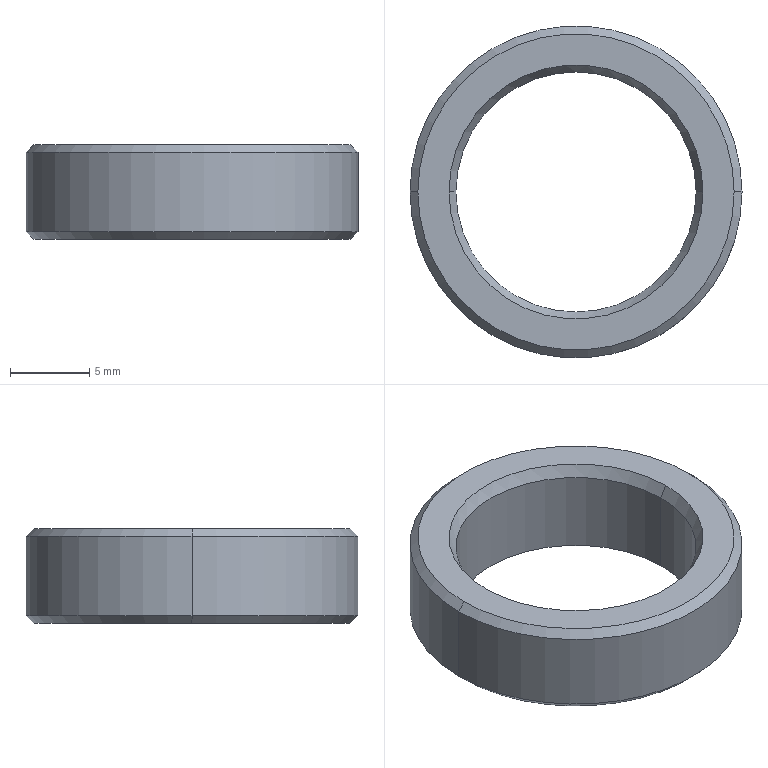Part | STEP file | ESPACIADOR POLEA 2 | 1 solid | 12 faces | box 21 x 21 x 6 mm | volume 965.28 mm3 | cone 6 | cylinder 4 | plane 2 | commonest cylinder face diameters 15.2 x2 21 x2
STEP:
#1=CARTESIAN_POINT('',(-7.6,0.,2.25));
#2=VERTEX_POINT('',#1);
#3=CARTESIAN_POINT('',(7.6,0.,2.25));
#4=VERTEX_POINT('',#3);
#5=CARTESIAN_POINT('',(0.,0.,2.25));
#6=DIRECTION('',(0.,0.,1.));
#7=DIRECTION('',(1.,0.,0.));
#8=AXIS2_PLACEMENT_3D('',#5,#6,#7);
#9=CIRCLE('',#8,7.6);
#10=EDGE_CURVE('',#2,#4,#9,.T.);
#11=ORIENTED_EDGE('',*,*,#10,.F.);
#12=CARTESIAN_POINT('',(-8.033,0.,3.));
#13=VERTEX_POINT('',#12);
#14=CARTESIAN_POINT('',(-7.6,0.,2.25));
#15=DIRECTION('',(-0.5,0.,0.866));
#16=VECTOR('',#15,1000.);
#17=LINE('',#14,#16);
#18=EDGE_CURVE('',#2,#13,#17,.T.);
#19=ORIENTED_EDGE('',*,*,#18,.T.);
#20=CARTESIAN_POINT('',(8.033,0.,3.));
#21=VERTEX_POINT('',#20);
#22=CARTESIAN_POINT('',(0.,0.,3.));
#23=DIRECTION('',(0.,0.,-1.));
#24=DIRECTION('',(1.,0.,0.));
#25=AXIS2_PLACEMENT_3D('',#22,#23,#24);
#26=CIRCLE('',#25,8.033);
#27=EDGE_CURVE('',#21,#13,#26,.T.);
#28=ORIENTED_EDGE('',*,*,#27,.F.);
#29=CARTESIAN_POINT('',(7.6,0.,2.25));
#30=DIRECTION('',(0.5,0.,0.866));
#31=VECTOR('',#30,1000.);
#32=LINE('',#29,#31);
#33=EDGE_CURVE('',#4,#21,#32,.T.);
#34=ORIENTED_EDGE('',*,*,#33,.F.);
#35=EDGE_LOOP('',(#11,#19,#28,#34));
#36=FACE_OUTER_BOUND('',#35,.T.);
#37=CARTESIAN_POINT('',(0.,0.,2.25));
#38=DIRECTION('',(0.,0.,1.));
#39=DIRECTION('',(1.,0.,0.));
#40=AXIS2_PLACEMENT_3D('',#37,#38,#39);
#41=CONICAL_SURFACE('',#40,7.6,0.5236);
#42=ADVANCED_FACE('',(#36),#41,.F.);
#43=CARTESIAN_POINT('',(10.,0.,3.));
#44=VERTEX_POINT('',#43);
#45=CARTESIAN_POINT('',(-10.,0.,3.));
#46=VERTEX_POINT('',#45);
#47=CARTESIAN_POINT('',(0.,0.,3.));
#48=DIRECTION('',(0.,0.,1.));
#49=DIRECTION('',(1.,0.,0.));
#50=AXIS2_PLACEMENT_3D('',#47,#48,#49);
#51=CIRCLE('',#50,10.);
#52=EDGE_CURVE('',#44,#46,#51,.T.);
#53=ORIENTED_EDGE('',*,*,#52,.F.);
#54=CARTESIAN_POINT('',(10.5,0.,2.5));
#55=VERTEX_POINT('',#54);
#56=CARTESIAN_POINT('',(10.,0.,3.));
#57=DIRECTION('',(0.7071,0.,-0.7071));
#58=VECTOR('',#57,1000.);
#59=LINE('',#56,#58);
#60=EDGE_CURVE('',#44,#55,#59,.T.);
#61=ORIENTED_EDGE('',*,*,#60,.T.);
#62=CARTESIAN_POINT('',(-10.5,0.,2.5));
#63=VERTEX_POINT('',#62);
#64=CARTESIAN_POINT('',(0.,0.,2.5));
#65=DIRECTION('',(0.,0.,-1.));
#66=DIRECTION('',(1.,0.,0.));
#67=AXIS2_PLACEMENT_3D('',#64,#65,#66);
#68=CIRCLE('',#67,10.5);
#69=EDGE_CURVE('',#63,#55,#68,.T.);
#70=ORIENTED_EDGE('',*,*,#69,.F.);
#71=CARTESIAN_POINT('',(-10.,0.,3.));
#72=DIRECTION('',(-0.7071,0.,-0.7071));
#73=VECTOR('',#72,1000.);
#74=LINE('',#71,#73);
#75=EDGE_CURVE('',#46,#63,#74,.T.);
#76=ORIENTED_EDGE('',*,*,#75,.F.);
#77=EDGE_LOOP('',(#53,#61,#70,#76));
#78=FACE_OUTER_BOUND('',#77,.T.);
#79=CARTESIAN_POINT('',(0.,0.,3.));
#80=DIRECTION('',(0.,0.,-1.));
#81=DIRECTION('',(-1.,0.,0.));
#82=AXIS2_PLACEMENT_3D('',#79,#80,#81);
#83=CONICAL_SURFACE('',#82,10.,0.7854);
#84=ADVANCED_FACE('',(#78),#83,.T.);
#85=CARTESIAN_POINT('',(-10.,0.,-3.));
#86=VERTEX_POINT('',#85);
#87=CARTESIAN_POINT('',(10.,0.,-3.));
#88=VERTEX_POINT('',#87);
#89=CARTESIAN_POINT('',(0.,0.,-3.));
#90=DIRECTION('',(0.,0.,-1.));
#91=DIRECTION('',(1.,0.,0.));
#92=AXIS2_PLACEMENT_3D('',#89,#90,#91);
#93=CIRCLE('',#92,10.);
#94=EDGE_CURVE('',#86,#88,#93,.T.);
#95=ORIENTED_EDGE('',*,*,#94,.F.);
#96=CARTESIAN_POINT('',(-10.5,0.,-2.5));
#97=VERTEX_POINT('',#96);
#98=CARTESIAN_POINT('',(-10.5,0.,-2.5));
#99=DIRECTION('',(-0.7071,0.,0.7071));
#100=VECTOR('',#99,1000.);
#101=LINE('',#98,#100);
#102=EDGE_CURVE('',#86,#97,#101,.T.);
#103=ORIENTED_EDGE('',*,*,#102,.T.);
#104=CARTESIAN_POINT('',(10.5,0.,-2.5));
#105=VERTEX_POINT('',#104);
#106=CARTESIAN_POINT('',(0.,0.,-2.5));
#107=DIRECTION('',(0.,0.,1.));
#108=DIRECTION('',(1.,0.,0.));
#109=AXIS2_PLACEMENT_3D('',#106,#107,#108);
#110=CIRCLE('',#109,10.5);
#111=EDGE_CURVE('',#105,#97,#110,.T.);
#112=ORIENTED_EDGE('',*,*,#111,.F.);
#113=CARTESIAN_POINT('',(10.5,0.,-2.5));
#114=DIRECTION('',(0.7071,0.,0.7071));
#115=VECTOR('',#114,1000.);
#116=LINE('',#113,#115);
#117=EDGE_CURVE('',#88,#105,#116,.T.);
#118=ORIENTED_EDGE('',*,*,#117,.F.);
#119=EDGE_LOOP('',(#95,#103,#112,#118));
#120=FACE_OUTER_BOUND('',#119,.T.);
#121=CARTESIAN_POINT('',(0.,0.,-2.5));
#122=DIRECTION('',(0.,0.,1.));
#123=DIRECTION('',(1.,0.,0.));
#124=AXIS2_PLACEMENT_3D('',#121,#122,#123);
#125=CONICAL_SURFACE('',#124,10.5,0.7854);
#126=ADVANCED_FACE('',(#120),#125,.T.);
#127=ORIENTED_EDGE('',*,*,#10,.T.);
#128=CARTESIAN_POINT('',(7.6,0.,-3.));
#129=VERTEX_POINT('',#128);
#130=CARTESIAN_POINT('',(7.6,0.,3.));
#131=DIRECTION('',(0.,0.,-1.));
#132=VECTOR('',#131,1000.);
#133=LINE('',#130,#132);
#134=EDGE_CURVE('',#4,#129,#133,.T.);
#135=ORIENTED_EDGE('',*,*,#134,.T.);
#136=CARTESIAN_POINT('',(-7.6,0.,-3.));
#137=VERTEX_POINT('',#136);
#138=CARTESIAN_POINT('',(0.,0.,-3.));
#139=DIRECTION('',(0.,0.,1.));
#140=DIRECTION('',(1.,0.,0.));
#141=AXIS2_PLACEMENT_3D('',#138,#139,#140);
#142=CIRCLE('',#141,7.6);
#143=EDGE_CURVE('',#137,#129,#142,.T.);
#144=ORIENTED_EDGE('',*,*,#143,.F.);
#145=CARTESIAN_POINT('',(-7.6,0.,3.));
#146=DIRECTION('',(0.,0.,-1.));
#147=VECTOR('',#146,1000.);
#148=LINE('',#145,#147);
#149=EDGE_CURVE('',#2,#137,#148,.T.);
#150=ORIENTED_EDGE('',*,*,#149,.F.);
#151=EDGE_LOOP('',(#127,#135,#144,#150));
#152=FACE_OUTER_BOUND('',#151,.T.);
#153=CARTESIAN_POINT('',(0.,0.,3.));
#154=DIRECTION('',(0.,0.,-1.));
#155=DIRECTION('',(-1.,0.,0.));
#156=AXIS2_PLACEMENT_3D('',#153,#154,#155);
#157=CYLINDRICAL_SURFACE('',#156,7.6);
#158=ADVANCED_FACE('',(#152),#157,.F.);
#159=ORIENTED_EDGE('',*,*,#69,.T.);
#160=CARTESIAN_POINT('',(10.5,0.,3.));
#161=DIRECTION('',(0.,0.,-1.));
#162=VECTOR('',#161,1000.);
#163=LINE('',#160,#162);
#164=EDGE_CURVE('',#55,#105,#163,.T.);
#165=ORIENTED_EDGE('',*,*,#164,.T.);
#166=ORIENTED_EDGE('',*,*,#111,.T.);
#167=CARTESIAN_POINT('',(-10.5,0.,3.));
#168=DIRECTION('',(0.,0.,-1.));
#169=VECTOR('',#168,1000.);
#170=LINE('',#167,#169);
#171=EDGE_CURVE('',#63,#97,#170,.T.);
#172=ORIENTED_EDGE('',*,*,#171,.F.);
#173=EDGE_LOOP('',(#159,#165,#166,#172));
#174=FACE_OUTER_BOUND('',#173,.T.);
#175=CARTESIAN_POINT('',(0.,0.,3.));
#176=DIRECTION('',(0.,0.,-1.));
#177=DIRECTION('',(-1.,0.,0.));
#178=AXIS2_PLACEMENT_3D('',#175,#176,#177);
#179=CYLINDRICAL_SURFACE('',#178,10.5);
#180=ADVANCED_FACE('',(#174),#179,.T.);
#181=ORIENTED_EDGE('',*,*,#27,.T.);
#182=CARTESIAN_POINT('',(0.,0.,3.));
#183=DIRECTION('',(0.,0.,-1.));
#184=DIRECTION('',(1.,0.,0.));
#185=AXIS2_PLACEMENT_3D('',#182,#183,#184);
#186=CIRCLE('',#185,8.033);
#187=EDGE_CURVE('',#13,#21,#186,.T.);
#188=ORIENTED_EDGE('',*,*,#187,.T.);
#189=EDGE_LOOP('',(#181,#188));
#190=FACE_BOUND('',#189,.T.);
#191=CARTESIAN_POINT('',(0.,0.,3.));
#192=DIRECTION('',(0.,0.,1.));
#193=DIRECTION('',(1.,0.,0.));
#194=AXIS2_PLACEMENT_3D('',#191,#192,#193);
#195=CIRCLE('',#194,10.);
#196=EDGE_CURVE('',#46,#44,#195,.T.);
#197=ORIENTED_EDGE('',*,*,#196,.T.);
#198=ORIENTED_EDGE('',*,*,#52,.T.);
#199=EDGE_LOOP('',(#197,#198));
#200=FACE_OUTER_BOUND('',#199,.T.);
#201=CARTESIAN_POINT('',(0.,0.,3.));
#202=DIRECTION('',(0.,0.,1.));
#203=DIRECTION('',(1.,0.,0.));
#204=AXIS2_PLACEMENT_3D('',#201,#202,#203);
#205=PLANE('',#204);
#206=ADVANCED_FACE('',(#190,#200),#205,.T.);
#207=CARTESIAN_POINT('',(0.,0.,-3.));
#208=DIRECTION('',(0.,0.,-1.));
#209=DIRECTION('',(1.,0.,0.));
#210=AXIS2_PLACEMENT_3D('',#207,#208,#209);
#211=CIRCLE('',#210,10.);
#212=EDGE_CURVE('',#88,#86,#211,.T.);
#213=ORIENTED_EDGE('',*,*,#212,.T.);
#214=ORIENTED_EDGE('',*,*,#94,.T.);
#215=EDGE_LOOP('',(#213,#214));
#216=FACE_OUTER_BOUND('',#215,.T.);
#217=ORIENTED_EDGE('',*,*,#143,.T.);
#218=CARTESIAN_POINT('',(0.,0.,-3.));
#219=DIRECTION('',(0.,0.,1.));
#220=DIRECTION('',(1.,0.,0.));
#221=AXIS2_PLACEMENT_3D('',#218,#219,#220);
#222=CIRCLE('',#221,7.6);
#223=EDGE_CURVE('',#129,#137,#222,.T.);
#224=ORIENTED_EDGE('',*,*,#223,.T.);
#225=EDGE_LOOP('',(#217,#224));
#226=FACE_BOUND('',#225,.T.);
#227=CARTESIAN_POINT('',(0.,0.,-3.));
#228=DIRECTION('',(0.,0.,1.));
#229=DIRECTION('',(1.,0.,0.));
#230=AXIS2_PLACEMENT_3D('',#227,#228,#229);
#231=PLANE('',#230);
#232=ADVANCED_FACE('',(#216,#226),#231,.F.);
#233=ORIENTED_EDGE('',*,*,#164,.F.);
#234=CARTESIAN_POINT('',(0.,0.,2.5));
#235=DIRECTION('',(0.,0.,-1.));
#236=DIRECTION('',(1.,0.,0.));
#237=AXIS2_PLACEMENT_3D('',#234,#235,#236);
#238=CIRCLE('',#237,10.5);
#239=EDGE_CURVE('',#55,#63,#238,.T.);
#240=ORIENTED_EDGE('',*,*,#239,.T.);
#241=ORIENTED_EDGE('',*,*,#171,.T.);
#242=CARTESIAN_POINT('',(0.,0.,-2.5));
#243=DIRECTION('',(0.,0.,1.));
#244=DIRECTION('',(1.,0.,0.));
#245=AXIS2_PLACEMENT_3D('',#242,#243,#244);
#246=CIRCLE('',#245,10.5);
#247=EDGE_CURVE('',#97,#105,#246,.T.);
#248=ORIENTED_EDGE('',*,*,#247,.T.);
#249=EDGE_LOOP('',(#233,#240,#241,#248));
#250=FACE_OUTER_BOUND('',#249,.T.);
#251=CARTESIAN_POINT('',(0.,0.,3.));
#252=DIRECTION('',(0.,0.,-1.));
#253=DIRECTION('',(-1.,0.,0.));
#254=AXIS2_PLACEMENT_3D('',#251,#252,#253);
#255=CYLINDRICAL_SURFACE('',#254,10.5);
#256=ADVANCED_FACE('',(#250),#255,.T.);
#257=ORIENTED_EDGE('',*,*,#134,.F.);
#258=CARTESIAN_POINT('',(0.,0.,2.25));
#259=DIRECTION('',(0.,0.,1.));
#260=DIRECTION('',(1.,0.,0.));
#261=AXIS2_PLACEMENT_3D('',#258,#259,#260);
#262=CIRCLE('',#261,7.6);
#263=EDGE_CURVE('',#4,#2,#262,.T.);
#264=ORIENTED_EDGE('',*,*,#263,.T.);
#265=ORIENTED_EDGE('',*,*,#149,.T.);
#266=ORIENTED_EDGE('',*,*,#223,.F.);
#267=EDGE_LOOP('',(#257,#264,#265,#266));
#268=FACE_OUTER_BOUND('',#267,.T.);
#269=CARTESIAN_POINT('',(0.,0.,3.));
#270=DIRECTION('',(0.,0.,-1.));
#271=DIRECTION('',(-1.,0.,0.));
#272=AXIS2_PLACEMENT_3D('',#269,#270,#271);
#273=CYLINDRICAL_SURFACE('',#272,7.6);
#274=ADVANCED_FACE('',(#268),#273,.F.);
#275=ORIENTED_EDGE('',*,*,#102,.F.);
#276=ORIENTED_EDGE('',*,*,#212,.F.);
#277=ORIENTED_EDGE('',*,*,#117,.T.);
#278=ORIENTED_EDGE('',*,*,#247,.F.);
#279=EDGE_LOOP('',(#275,#276,#277,#278));
#280=FACE_OUTER_BOUND('',#279,.T.);
#281=CARTESIAN_POINT('',(0.,0.,-2.5));
#282=DIRECTION('',(0.,0.,1.));
#283=DIRECTION('',(1.,0.,0.));
#284=AXIS2_PLACEMENT_3D('',#281,#282,#283);
#285=CONICAL_SURFACE('',#284,10.5,0.7854);
#286=ADVANCED_FACE('',(#280),#285,.T.);
#287=ORIENTED_EDGE('',*,*,#60,.F.);
#288=ORIENTED_EDGE('',*,*,#196,.F.);
#289=ORIENTED_EDGE('',*,*,#75,.T.);
#290=ORIENTED_EDGE('',*,*,#239,.F.);
#291=EDGE_LOOP('',(#287,#288,#289,#290));
#292=FACE_OUTER_BOUND('',#291,.T.);
#293=CARTESIAN_POINT('',(0.,0.,3.));
#294=DIRECTION('',(0.,0.,-1.));
#295=DIRECTION('',(-1.,0.,0.));
#296=AXIS2_PLACEMENT_3D('',#293,#294,#295);
#297=CONICAL_SURFACE('',#296,10.,0.7854);
#298=ADVANCED_FACE('',(#292),#297,.T.);
#299=ORIENTED_EDGE('',*,*,#18,.F.);
#300=ORIENTED_EDGE('',*,*,#263,.F.);
#301=ORIENTED_EDGE('',*,*,#33,.T.);
#302=ORIENTED_EDGE('',*,*,#187,.F.);
#303=EDGE_LOOP('',(#299,#300,#301,#302));
#304=FACE_OUTER_BOUND('',#303,.T.);
#305=CARTESIAN_POINT('',(0.,0.,2.25));
#306=DIRECTION('',(0.,0.,1.));
#307=DIRECTION('',(1.,0.,0.));
#308=AXIS2_PLACEMENT_3D('',#305,#306,#307);
#309=CONICAL_SURFACE('',#308,7.6,0.5236);
#310=ADVANCED_FACE('',(#304),#309,.F.);
#311=CLOSED_SHELL('',(#42,#84,#126,#158,#180,#206,#232,#256,#274,#286,#298,#310));
#312=MANIFOLD_SOLID_BREP('',#311);
#313=CARTESIAN_POINT('',(0.,0.,0.));
#314=DIRECTION('',(0.,0.,1.));
#315=DIRECTION('',(1.,0.,0.));
#316=AXIS2_PLACEMENT_3D('',#313,#314,#315);
#317=(LENGTH_UNIT()NAMED_UNIT(*)SI_UNIT(.MILLI.,.METRE.));
#318=UNCERTAINTY_MEASURE_WITH_UNIT(LENGTH_MEASURE(0.00001),#317,'','');
#319=(NAMED_UNIT(*)PLANE_ANGLE_UNIT()SI_UNIT($,.RADIAN.));
#320=(NAMED_UNIT(*)SI_UNIT($,.STERADIAN.)SOLID_ANGLE_UNIT());
#321=(GEOMETRIC_REPRESENTATION_CONTEXT(3)GLOBAL_UNCERTAINTY_ASSIGNED_CONTEXT((#318))GLOBAL_UNIT_ASSIGNED_CONTEXT((#317,#319,#320))REPRESENTATION_CONTEXT('',''));
#322=ADVANCED_BREP_SHAPE_REPRESENTATION('',(#312,#316),#321);